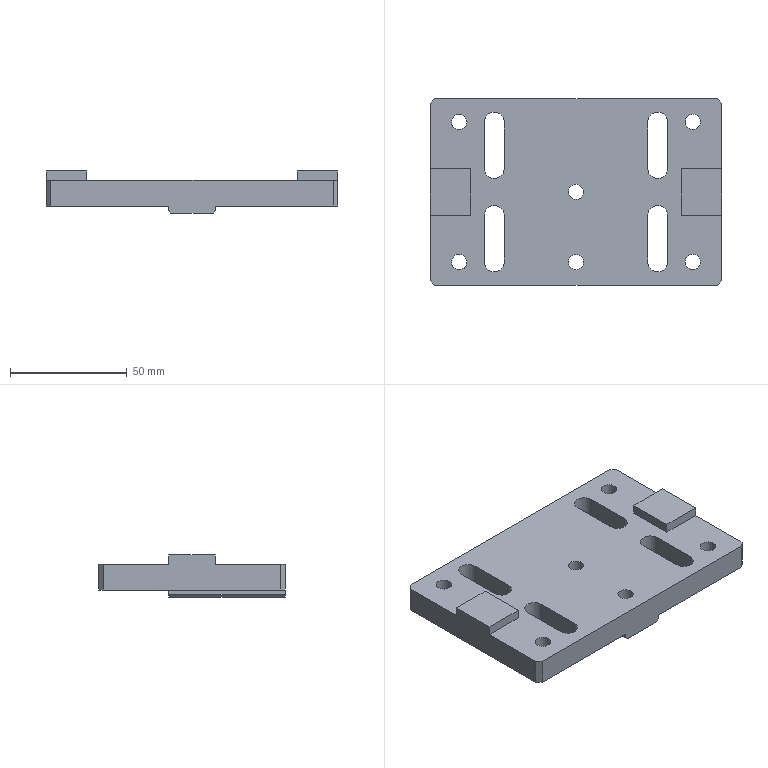Part | 1 solid | 54 faces | box 125 x 80 x 18 mm | volume 101791 mm3 | plane 36 | cylinder 18 | commonest cylinder face diameters 8.5 x8 6.6 x4 11 x4 6.5 x2